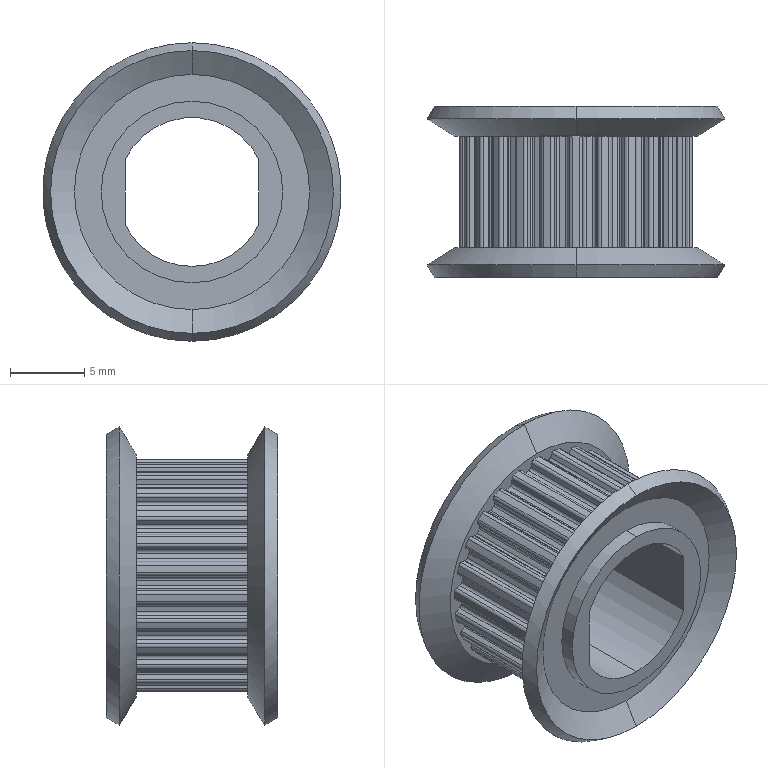Part | NX | features BREP 1 | 1 solid | 247 faces | box 20.061 x 11.5 x 20.061 mm | volume 1335 mm3 | cylinder 152 | plane 83 | cone 12 | commonest cylinder face diameters 0.46 x120 15.66 x25 12.2 x4 10 x3